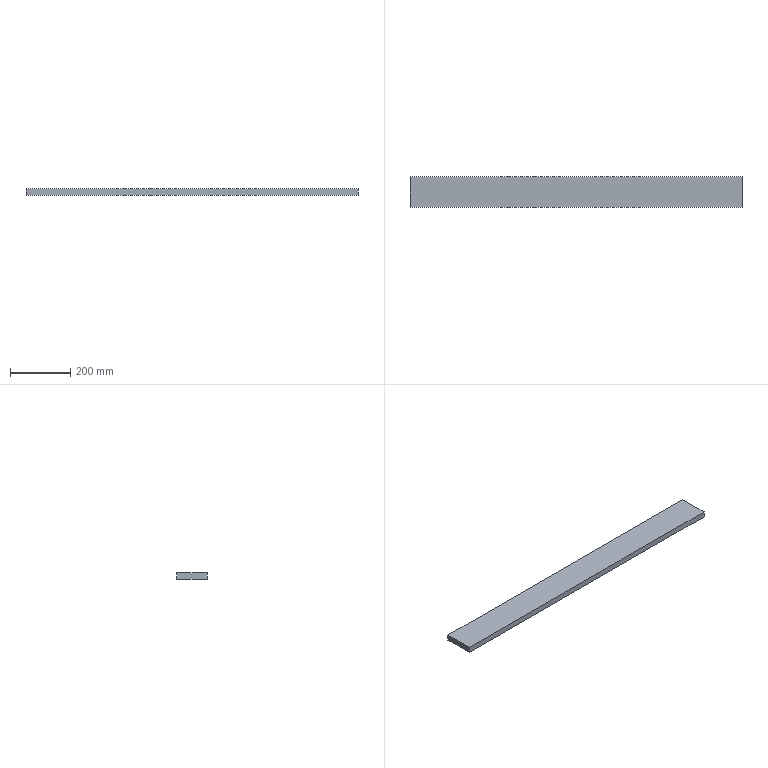Part | SolidWorks | features Extrusion 1 | 1 solid | 6 faces | box 1100 x 100 x 20 mm | volume 2200000 mm3 | plane 6
STEP:
#1=CARTESIAN_POINT('',(0.,100.,0.));
#2=VERTEX_POINT('',#1);
#3=CARTESIAN_POINT('',(0.,0.,0.));
#4=VERTEX_POINT('',#3);
#5=CARTESIAN_POINT('',(0.,0.,0.));
#6=DIRECTION('',(0.,-1.,0.));
#7=VECTOR('',#6,1000.);
#8=LINE('',#5,#7);
#9=EDGE_CURVE('',#2,#4,#8,.T.);
#10=ORIENTED_EDGE('',*,*,#9,.T.);
#11=CARTESIAN_POINT('',(0.,0.,20.));
#12=VERTEX_POINT('',#11);
#13=CARTESIAN_POINT('',(0.,0.,20.));
#14=DIRECTION('',(0.,0.,-1.));
#15=VECTOR('',#14,1000.);
#16=LINE('',#13,#15);
#17=EDGE_CURVE('',#12,#4,#16,.T.);
#18=ORIENTED_EDGE('',*,*,#17,.F.);
#19=CARTESIAN_POINT('',(0.,100.,20.));
#20=VERTEX_POINT('',#19);
#21=CARTESIAN_POINT('',(0.,0.,20.));
#22=DIRECTION('',(0.,-1.,0.));
#23=VECTOR('',#22,1000.);
#24=LINE('',#21,#23);
#25=EDGE_CURVE('',#20,#12,#24,.T.);
#26=ORIENTED_EDGE('',*,*,#25,.F.);
#27=CARTESIAN_POINT('',(0.,100.,20.));
#28=DIRECTION('',(0.,0.,-1.));
#29=VECTOR('',#28,1000.);
#30=LINE('',#27,#29);
#31=EDGE_CURVE('',#20,#2,#30,.T.);
#32=ORIENTED_EDGE('',*,*,#31,.T.);
#33=EDGE_LOOP('',(#10,#18,#26,#32));
#34=FACE_OUTER_BOUND('',#33,.T.);
#35=CARTESIAN_POINT('',(0.,0.,20.));
#36=DIRECTION('',(1.,0.,0.));
#37=DIRECTION('',(0.,0.,-1.));
#38=AXIS2_PLACEMENT_3D('',#35,#36,#37);
#39=PLANE('',#38);
#40=ADVANCED_FACE('',(#34),#39,.F.);
#41=CARTESIAN_POINT('',(1100.,0.,0.));
#42=VERTEX_POINT('',#41);
#43=CARTESIAN_POINT('',(0.,0.,0.));
#44=DIRECTION('',(1.,0.,0.));
#45=VECTOR('',#44,1000.);
#46=LINE('',#43,#45);
#47=EDGE_CURVE('',#4,#42,#46,.T.);
#48=ORIENTED_EDGE('',*,*,#47,.T.);
#49=CARTESIAN_POINT('',(1100.,0.,20.));
#50=VERTEX_POINT('',#49);
#51=CARTESIAN_POINT('',(1100.,0.,20.));
#52=DIRECTION('',(0.,0.,-1.));
#53=VECTOR('',#52,1000.);
#54=LINE('',#51,#53);
#55=EDGE_CURVE('',#50,#42,#54,.T.);
#56=ORIENTED_EDGE('',*,*,#55,.F.);
#57=CARTESIAN_POINT('',(0.,0.,20.));
#58=DIRECTION('',(1.,0.,0.));
#59=VECTOR('',#58,1000.);
#60=LINE('',#57,#59);
#61=EDGE_CURVE('',#12,#50,#60,.T.);
#62=ORIENTED_EDGE('',*,*,#61,.F.);
#63=ORIENTED_EDGE('',*,*,#17,.T.);
#64=EDGE_LOOP('',(#48,#56,#62,#63));
#65=FACE_OUTER_BOUND('',#64,.T.);
#66=CARTESIAN_POINT('',(0.,0.,20.));
#67=DIRECTION('',(0.,1.,0.));
#68=DIRECTION('',(0.,0.,1.));
#69=AXIS2_PLACEMENT_3D('',#66,#67,#68);
#70=PLANE('',#69);
#71=ADVANCED_FACE('',(#65),#70,.F.);
#72=CARTESIAN_POINT('',(1100.,100.,0.));
#73=VERTEX_POINT('',#72);
#74=CARTESIAN_POINT('',(1100.,0.,0.));
#75=DIRECTION('',(0.,1.,0.));
#76=VECTOR('',#75,1000.);
#77=LINE('',#74,#76);
#78=EDGE_CURVE('',#42,#73,#77,.T.);
#79=ORIENTED_EDGE('',*,*,#78,.T.);
#80=CARTESIAN_POINT('',(1100.,100.,20.));
#81=VERTEX_POINT('',#80);
#82=CARTESIAN_POINT('',(1100.,100.,20.));
#83=DIRECTION('',(0.,0.,-1.));
#84=VECTOR('',#83,1000.);
#85=LINE('',#82,#84);
#86=EDGE_CURVE('',#81,#73,#85,.T.);
#87=ORIENTED_EDGE('',*,*,#86,.F.);
#88=CARTESIAN_POINT('',(1100.,0.,20.));
#89=DIRECTION('',(0.,1.,0.));
#90=VECTOR('',#89,1000.);
#91=LINE('',#88,#90);
#92=EDGE_CURVE('',#50,#81,#91,.T.);
#93=ORIENTED_EDGE('',*,*,#92,.F.);
#94=ORIENTED_EDGE('',*,*,#55,.T.);
#95=EDGE_LOOP('',(#79,#87,#93,#94));
#96=FACE_OUTER_BOUND('',#95,.T.);
#97=CARTESIAN_POINT('',(1100.,0.,20.));
#98=DIRECTION('',(-1.,0.,0.));
#99=DIRECTION('',(0.,0.,1.));
#100=AXIS2_PLACEMENT_3D('',#97,#98,#99);
#101=PLANE('',#100);
#102=ADVANCED_FACE('',(#96),#101,.F.);
#103=CARTESIAN_POINT('',(0.,100.,0.));
#104=DIRECTION('',(-1.,0.,0.));
#105=VECTOR('',#104,1000.);
#106=LINE('',#103,#105);
#107=EDGE_CURVE('',#73,#2,#106,.T.);
#108=ORIENTED_EDGE('',*,*,#107,.T.);
#109=ORIENTED_EDGE('',*,*,#31,.F.);
#110=CARTESIAN_POINT('',(0.,100.,20.));
#111=DIRECTION('',(-1.,0.,0.));
#112=VECTOR('',#111,1000.);
#113=LINE('',#110,#112);
#114=EDGE_CURVE('',#81,#20,#113,.T.);
#115=ORIENTED_EDGE('',*,*,#114,.F.);
#116=ORIENTED_EDGE('',*,*,#86,.T.);
#117=EDGE_LOOP('',(#108,#109,#115,#116));
#118=FACE_OUTER_BOUND('',#117,.T.);
#119=CARTESIAN_POINT('',(0.,100.,20.));
#120=DIRECTION('',(0.,-1.,0.));
#121=DIRECTION('',(0.,0.,-1.));
#122=AXIS2_PLACEMENT_3D('',#119,#120,#121);
#123=PLANE('',#122);
#124=ADVANCED_FACE('',(#118),#123,.F.);
#125=ORIENTED_EDGE('',*,*,#25,.T.);
#126=ORIENTED_EDGE('',*,*,#61,.T.);
#127=ORIENTED_EDGE('',*,*,#92,.T.);
#128=ORIENTED_EDGE('',*,*,#114,.T.);
#129=EDGE_LOOP('',(#125,#126,#127,#128));
#130=FACE_OUTER_BOUND('',#129,.T.);
#131=CARTESIAN_POINT('',(0.,0.,20.));
#132=DIRECTION('',(0.,0.,-1.));
#133=DIRECTION('',(-1.,0.,0.));
#134=AXIS2_PLACEMENT_3D('',#131,#132,#133);
#135=PLANE('',#134);
#136=ADVANCED_FACE('',(#130),#135,.F.);
#137=ORIENTED_EDGE('',*,*,#9,.F.);
#138=ORIENTED_EDGE('',*,*,#107,.F.);
#139=ORIENTED_EDGE('',*,*,#78,.F.);
#140=ORIENTED_EDGE('',*,*,#47,.F.);
#141=EDGE_LOOP('',(#137,#138,#139,#140));
#142=FACE_OUTER_BOUND('',#141,.T.);
#143=CARTESIAN_POINT('',(0.,0.,0.));
#144=DIRECTION('',(0.,0.,-1.));
#145=DIRECTION('',(-1.,0.,0.));
#146=AXIS2_PLACEMENT_3D('',#143,#144,#145);
#147=PLANE('',#146);
#148=ADVANCED_FACE('',(#142),#147,.T.);
#149=CLOSED_SHELL('',(#40,#71,#102,#124,#136,#148));
#150=MANIFOLD_SOLID_BREP('',#149);
#151=CARTESIAN_POINT('',(0.,0.,0.));
#152=DIRECTION('',(0.,0.,1.));
#153=DIRECTION('',(1.,0.,0.));
#154=AXIS2_PLACEMENT_3D('',#151,#152,#153);
#155=(LENGTH_UNIT()NAMED_UNIT(*)SI_UNIT(.MILLI.,.METRE.));
#156=UNCERTAINTY_MEASURE_WITH_UNIT(LENGTH_MEASURE(0.00001),#155,'','');
#157=(NAMED_UNIT(*)PLANE_ANGLE_UNIT()SI_UNIT($,.RADIAN.));
#158=(NAMED_UNIT(*)SI_UNIT($,.STERADIAN.)SOLID_ANGLE_UNIT());
#159=(GEOMETRIC_REPRESENTATION_CONTEXT(3)GLOBAL_UNCERTAINTY_ASSIGNED_CONTEXT((#156))GLOBAL_UNIT_ASSIGNED_CONTEXT((#155,#157,#158))REPRESENTATION_CONTEXT('',''));
#160=ADVANCED_BREP_SHAPE_REPRESENTATION('',(#150,#154),#159);